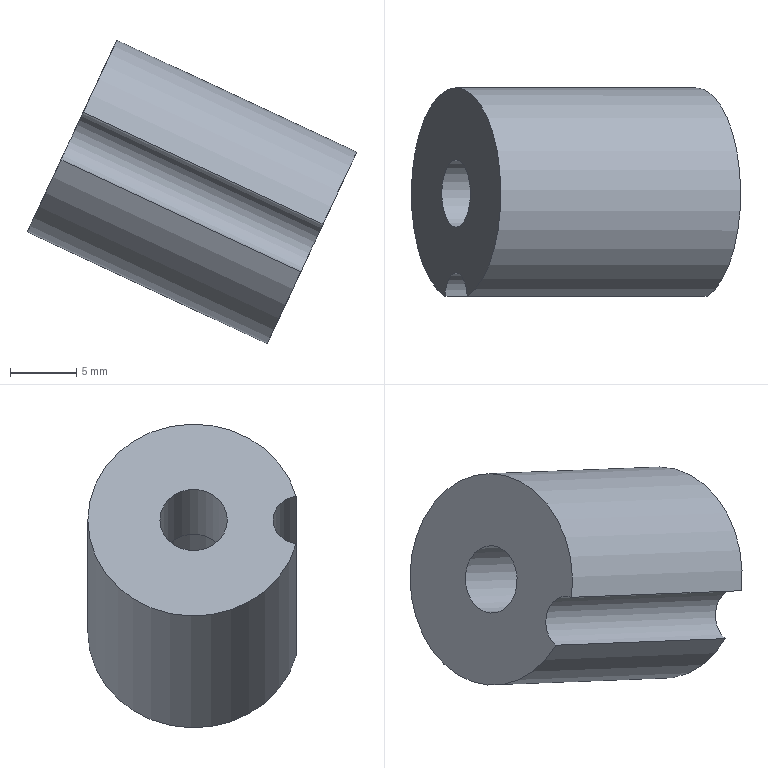Part | NX | features solid 2 | 1 solid | 7 faces | box 24.888 x 15.75 x 22.953 mm | volume 2680 mm3 | cylinder 4 | plane 3 | commonest cylinder face diameters 4 x1 5.1 x1 10.6 x1 16 x1
STEP:
#1=CARTESIAN_POINT('',(-593.923,-334.215,48.495));
#2=VERTEX_POINT('',#1);
#3=CARTESIAN_POINT('',(-612.049,-334.215,56.948));
#4=VERTEX_POINT('',#3);
#5=CARTESIAN_POINT('',(-602.986,-334.215,52.722));
#6=DIRECTION('',(-0.9063,0.,0.4226));
#7=VECTOR('',#6,1000.);
#8=LINE('',#5,#7);
#9=EDGE_CURVE('',#2,#4,#8,.T.);
#10=ORIENTED_EDGE('',*,*,#9,.F.);
#11=CARTESIAN_POINT('',(-595.6,-334.215,44.899));
#12=VERTEX_POINT('',#11);
#13=CARTESIAN_POINT('',(-594.762,-326.465,46.697));
#14=DIRECTION('',(-0.9063,0.,0.4226));
#15=DIRECTION('',(0.,-1.,0.));
#16=AXIS2_PLACEMENT_3D('',#13,#14,#15);
#17=CIRCLE('',#16,8.);
#18=EDGE_CURVE('',#2,#12,#17,.T.);
#19=ORIENTED_EDGE('',*,*,#18,.T.);
#20=CARTESIAN_POINT('',(-613.726,-334.215,53.351));
#21=VERTEX_POINT('',#20);
#22=CARTESIAN_POINT('',(-604.663,-334.215,49.125));
#23=DIRECTION('',(-0.9063,0.,0.4226));
#24=VECTOR('',#23,1000.);
#25=LINE('',#22,#24);
#26=EDGE_CURVE('',#21,#12,#25,.F.);
#27=ORIENTED_EDGE('',*,*,#26,.F.);
#28=CARTESIAN_POINT('',(-612.888,-326.465,55.149));
#29=DIRECTION('',(-0.9063,0.,0.4226));
#30=DIRECTION('',(0.,-1.,0.));
#31=AXIS2_PLACEMENT_3D('',#28,#29,#30);
#32=CIRCLE('',#31,8.);
#33=EDGE_CURVE('',#4,#21,#32,.T.);
#34=ORIENTED_EDGE('',*,*,#33,.F.);
#35=EDGE_LOOP('',(#10,#19,#27,#34));
#36=FACE_BOUND('',#35,.T.);
#37=CARTESIAN_POINT('',(-594.762,-326.465,46.697));
#38=DIRECTION('',(-0.9063,0.,0.4226));
#39=DIRECTION('',(0.,-1.,0.));
#40=AXIS2_PLACEMENT_3D('',#37,#38,#39);
#41=CYLINDRICAL_SURFACE('',#40,8.);
#42=ADVANCED_FACE('',(#36),#41,.T.);
#43=CARTESIAN_POINT('',(-594.762,-331.765,46.697));
#44=VERTEX_POINT('',#43);
#45=CARTESIAN_POINT('',(-594.762,-326.465,46.697));
#46=DIRECTION('',(-0.9063,0.,0.4226));
#47=DIRECTION('',(0.,-1.,0.));
#48=AXIS2_PLACEMENT_3D('',#45,#46,#47);
#49=CIRCLE('',#48,5.3);
#50=EDGE_CURVE('',#44,#44,#49,.T.);
#51=ORIENTED_EDGE('',*,*,#50,.T.);
#52=EDGE_LOOP('',(#51));
#53=FACE_BOUND('',#52,.T.);
#54=ORIENTED_EDGE('',*,*,#18,.F.);
#55=CARTESIAN_POINT('',(-594.762,-334.465,46.697));
#56=DIRECTION('',(-0.9063,0.,0.4226));
#57=DIRECTION('',(0.,-1.,0.));
#58=AXIS2_PLACEMENT_3D('',#55,#56,#57);
#59=CIRCLE('',#58,2.);
#60=EDGE_CURVE('',#2,#12,#59,.T.);
#61=ORIENTED_EDGE('',*,*,#60,.T.);
#62=EDGE_LOOP('',(#54,#61));
#63=FACE_BOUND('',#62,.T.);
#64=CARTESIAN_POINT('',(-594.762,-326.465,46.697));
#65=DIRECTION('',(-0.9063,0.,0.4226));
#66=DIRECTION('',(0.,-1.,0.));
#67=AXIS2_PLACEMENT_3D('',#64,#65,#66);
#68=PLANE('',#67);
#69=ADVANCED_FACE('',(#53,#63),#68,.F.);
#70=CARTESIAN_POINT('',(-612.888,-329.015,55.149));
#71=VERTEX_POINT('',#70);
#72=CARTESIAN_POINT('',(-612.888,-326.465,55.149));
#73=DIRECTION('',(-0.9063,0.,0.4226));
#74=DIRECTION('',(0.,-1.,0.));
#75=AXIS2_PLACEMENT_3D('',#72,#73,#74);
#76=CIRCLE('',#75,2.55);
#77=EDGE_CURVE('',#71,#71,#76,.T.);
#78=ORIENTED_EDGE('',*,*,#77,.F.);
#79=EDGE_LOOP('',(#78));
#80=FACE_BOUND('',#79,.T.);
#81=CARTESIAN_POINT('',(-612.888,-334.465,55.149));
#82=DIRECTION('',(-0.9063,0.,0.4226));
#83=DIRECTION('',(0.,-1.,0.));
#84=AXIS2_PLACEMENT_3D('',#81,#82,#83);
#85=CIRCLE('',#84,2.);
#86=EDGE_CURVE('',#4,#21,#85,.T.);
#87=ORIENTED_EDGE('',*,*,#86,.F.);
#88=ORIENTED_EDGE('',*,*,#33,.T.);
#89=EDGE_LOOP('',(#87,#88));
#90=FACE_BOUND('',#89,.T.);
#91=CARTESIAN_POINT('',(-612.888,-326.465,55.149));
#92=DIRECTION('',(-0.9063,0.,0.4226));
#93=DIRECTION('',(0.,-1.,0.));
#94=AXIS2_PLACEMENT_3D('',#91,#92,#93);
#95=PLANE('',#94);
#96=ADVANCED_FACE('',(#80,#90),#95,.T.);
#97=ORIENTED_EDGE('',*,*,#50,.F.);
#98=EDGE_LOOP('',(#97));
#99=FACE_BOUND('',#98,.T.);
#100=CARTESIAN_POINT('',(-605.637,-331.765,51.768));
#101=VERTEX_POINT('',#100);
#102=CARTESIAN_POINT('',(-605.637,-326.465,51.768));
#103=DIRECTION('',(-0.9063,0.,0.4226));
#104=DIRECTION('',(0.,-1.,0.));
#105=AXIS2_PLACEMENT_3D('',#102,#103,#104);
#106=CIRCLE('',#105,5.3);
#107=EDGE_CURVE('',#101,#101,#106,.T.);
#108=ORIENTED_EDGE('',*,*,#107,.T.);
#109=EDGE_LOOP('',(#108));
#110=FACE_BOUND('',#109,.T.);
#111=CARTESIAN_POINT('',(-594.762,-326.465,46.697));
#112=DIRECTION('',(-0.9063,0.,0.4226));
#113=DIRECTION('',(0.,-1.,0.));
#114=AXIS2_PLACEMENT_3D('',#111,#112,#113);
#115=CYLINDRICAL_SURFACE('',#114,5.3);
#116=ADVANCED_FACE('',(#99,#110),#115,.F.);
#117=CARTESIAN_POINT('',(-605.637,-329.015,51.768));
#118=VERTEX_POINT('',#117);
#119=CARTESIAN_POINT('',(-605.637,-326.465,51.768));
#120=DIRECTION('',(-0.9063,0.,0.4226));
#121=DIRECTION('',(0.,-1.,0.));
#122=AXIS2_PLACEMENT_3D('',#119,#120,#121);
#123=CIRCLE('',#122,2.55);
#124=EDGE_CURVE('',#118,#118,#123,.T.);
#125=ORIENTED_EDGE('',*,*,#124,.T.);
#126=EDGE_LOOP('',(#125));
#127=FACE_BOUND('',#126,.T.);
#128=ORIENTED_EDGE('',*,*,#107,.F.);
#129=EDGE_LOOP('',(#128));
#130=FACE_BOUND('',#129,.T.);
#131=CARTESIAN_POINT('',(-605.637,-326.465,51.768));
#132=DIRECTION('',(-0.9063,0.,0.4226));
#133=DIRECTION('',(0.,-1.,0.));
#134=AXIS2_PLACEMENT_3D('',#131,#132,#133);
#135=PLANE('',#134);
#136=ADVANCED_FACE('',(#127,#130),#135,.F.);
#137=ORIENTED_EDGE('',*,*,#9,.T.);
#138=ORIENTED_EDGE('',*,*,#86,.T.);
#139=ORIENTED_EDGE('',*,*,#26,.T.);
#140=ORIENTED_EDGE('',*,*,#60,.F.);
#141=EDGE_LOOP('',(#137,#138,#139,#140));
#142=FACE_BOUND('',#141,.T.);
#143=CARTESIAN_POINT('',(-594.762,-334.465,46.697));
#144=DIRECTION('',(-0.9063,0.,0.4226));
#145=DIRECTION('',(0.,-1.,0.));
#146=AXIS2_PLACEMENT_3D('',#143,#144,#145);
#147=CYLINDRICAL_SURFACE('',#146,2.);
#148=ADVANCED_FACE('',(#142),#147,.F.);
#149=ORIENTED_EDGE('',*,*,#77,.T.);
#150=EDGE_LOOP('',(#149));
#151=FACE_BOUND('',#150,.T.);
#152=ORIENTED_EDGE('',*,*,#124,.F.);
#153=EDGE_LOOP('',(#152));
#154=FACE_BOUND('',#153,.T.);
#155=CARTESIAN_POINT('',(-594.762,-326.465,46.697));
#156=DIRECTION('',(-0.9063,0.,0.4226));
#157=DIRECTION('',(0.,-1.,0.));
#158=AXIS2_PLACEMENT_3D('',#155,#156,#157);
#159=CYLINDRICAL_SURFACE('',#158,2.55);
#160=ADVANCED_FACE('',(#151,#154),#159,.F.);
#161=CLOSED_SHELL('',(#42,#69,#96,#116,#136,#148,#160));
#162=MANIFOLD_SOLID_BREP('',#161);
#163=(LENGTH_UNIT()NAMED_UNIT(*)SI_UNIT(.MILLI.,.METRE.));
#164=UNCERTAINTY_MEASURE_WITH_UNIT(LENGTH_MEASURE(0.00001),#163,'','');
#165=(NAMED_UNIT(*)PLANE_ANGLE_UNIT()SI_UNIT($,.RADIAN.));
#166=(NAMED_UNIT(*)SI_UNIT($,.STERADIAN.)SOLID_ANGLE_UNIT());
#167=(GEOMETRIC_REPRESENTATION_CONTEXT(3)GLOBAL_UNCERTAINTY_ASSIGNED_CONTEXT((#164))GLOBAL_UNIT_ASSIGNED_CONTEXT((#163,#165,#166))REPRESENTATION_CONTEXT('',''));
#168=ADVANCED_BREP_SHAPE_REPRESENTATION('',(#162),#167);